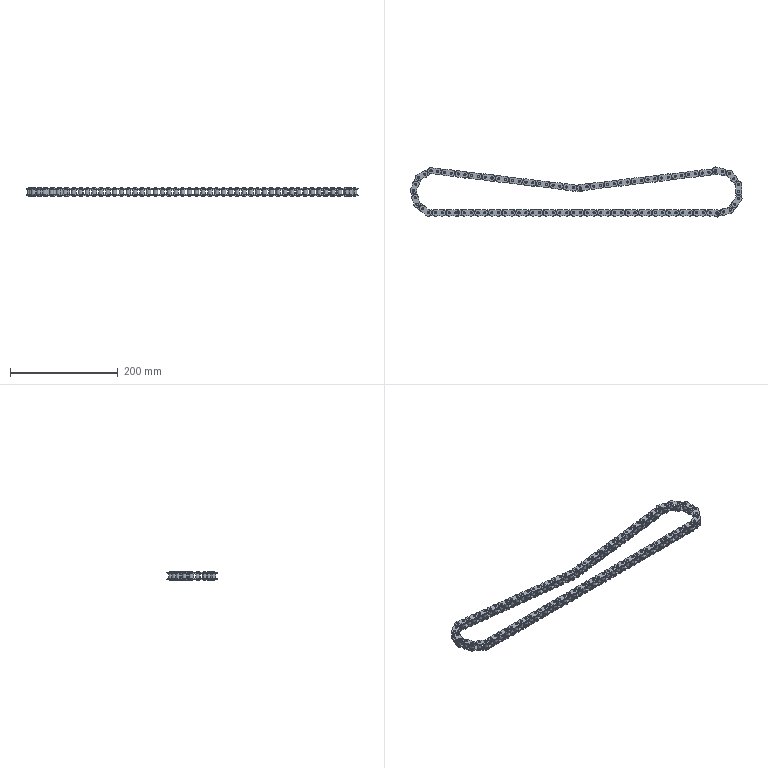Part | STEP file | Middle chain 2 | 153 solids | 3060 faces | volume 129311 mm3 | cylinder 2040 | plane 612 | cone 408 | commonest cylinder face diameters 3.98 x816 12.07 x612 55.348 x408 7.92 x204